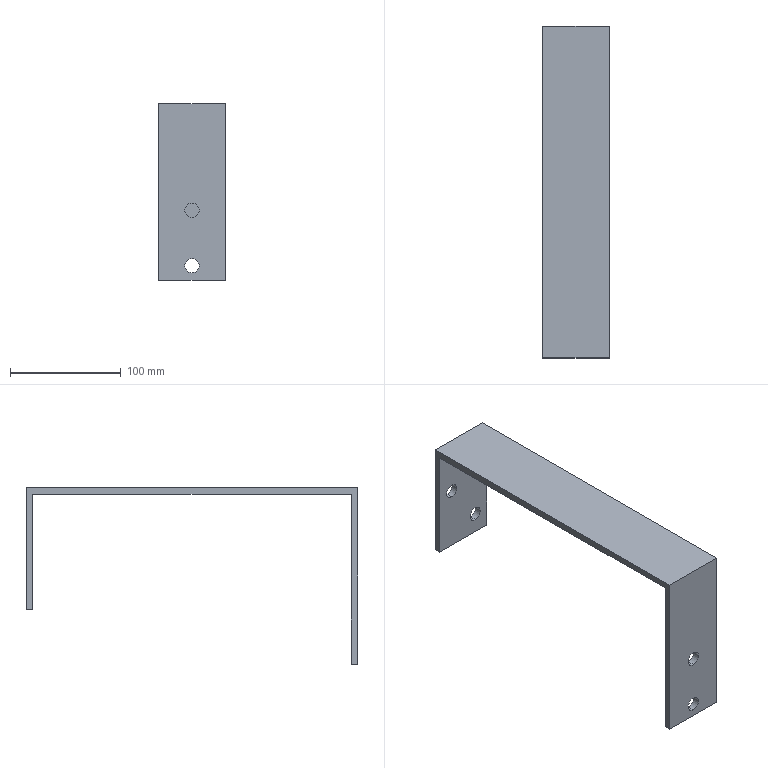Part | SolidWorks | features BaseBody 1 | 1 solid | 18 faces | box 60 x 299 x 159 mm | volume 196974 mm3 | plane 10 | cylinder 8 | commonest cylinder face diameters 13 x8
STEP:
#1=CARTESIAN_POINT('',(561.946,-3187.473,1586.471));
#2=VERTEX_POINT('',#1);
#3=CARTESIAN_POINT('',(561.946,-3187.473,1573.471));
#4=VERTEX_POINT('',#3);
#5=CARTESIAN_POINT('',(561.946,-3187.473,1579.971));
#6=DIRECTION('',(0.,-1.,0.));
#7=DIRECTION('',(0.,0.,-1.));
#8=AXIS2_PLACEMENT_3D('',#5,#6,#7);
#9=CIRCLE('',#8,6.5);
#10=EDGE_CURVE('',#2,#4,#9,.T.);
#11=ORIENTED_EDGE('',*,*,#10,.F.);
#12=CARTESIAN_POINT('',(561.946,-3193.473,1586.471));
#13=VERTEX_POINT('',#12);
#14=CARTESIAN_POINT('',(561.946,-3199.794,1586.471));
#15=DIRECTION('',(0.,-1.,0.));
#16=VECTOR('',#15,1000.);
#17=LINE('',#14,#16);
#18=EDGE_CURVE('',#2,#13,#17,.T.);
#19=ORIENTED_EDGE('',*,*,#18,.T.);
#20=CARTESIAN_POINT('',(561.946,-3193.473,1573.471));
#21=VERTEX_POINT('',#20);
#22=CARTESIAN_POINT('',(561.946,-3193.473,1579.971));
#23=DIRECTION('',(0.,1.,0.));
#24=DIRECTION('',(0.,0.,-1.));
#25=AXIS2_PLACEMENT_3D('',#22,#23,#24);
#26=CIRCLE('',#25,6.5);
#27=EDGE_CURVE('',#21,#13,#26,.T.);
#28=ORIENTED_EDGE('',*,*,#27,.F.);
#29=CARTESIAN_POINT('',(561.946,-3199.794,1573.471));
#30=DIRECTION('',(0.,-1.,0.));
#31=VECTOR('',#30,1000.);
#32=LINE('',#29,#31);
#33=EDGE_CURVE('',#4,#21,#32,.T.);
#34=ORIENTED_EDGE('',*,*,#33,.F.);
#35=EDGE_LOOP('',(#11,#19,#28,#34));
#36=FACE_OUTER_BOUND('',#35,.T.);
#37=CARTESIAN_POINT('',(561.946,-3199.794,1579.971));
#38=DIRECTION('',(0.,-1.,0.));
#39=DIRECTION('',(0.,0.,-1.));
#40=AXIS2_PLACEMENT_3D('',#37,#38,#39);
#41=CYLINDRICAL_SURFACE('',#40,6.5);
#42=ADVANCED_FACE('',(#36),#41,.F.);
#43=CARTESIAN_POINT('',(531.946,-3187.473,1626.471));
#44=VERTEX_POINT('',#43);
#45=CARTESIAN_POINT('',(531.946,-3187.473,1613.471));
#46=VERTEX_POINT('',#45);
#47=CARTESIAN_POINT('',(531.946,-3187.473,1619.971));
#48=DIRECTION('',(0.,-1.,0.));
#49=DIRECTION('',(0.,0.,-1.));
#50=AXIS2_PLACEMENT_3D('',#47,#48,#49);
#51=CIRCLE('',#50,6.5);
#52=EDGE_CURVE('',#44,#46,#51,.T.);
#53=ORIENTED_EDGE('',*,*,#52,.F.);
#54=CARTESIAN_POINT('',(531.946,-3193.473,1626.471));
#55=VERTEX_POINT('',#54);
#56=CARTESIAN_POINT('',(531.946,-3213.972,1626.471));
#57=DIRECTION('',(0.,-1.,0.));
#58=VECTOR('',#57,1000.);
#59=LINE('',#56,#58);
#60=EDGE_CURVE('',#44,#55,#59,.T.);
#61=ORIENTED_EDGE('',*,*,#60,.T.);
#62=CARTESIAN_POINT('',(531.946,-3193.473,1613.471));
#63=VERTEX_POINT('',#62);
#64=CARTESIAN_POINT('',(531.946,-3193.473,1619.971));
#65=DIRECTION('',(0.,1.,0.));
#66=DIRECTION('',(0.,0.,-1.));
#67=AXIS2_PLACEMENT_3D('',#64,#65,#66);
#68=CIRCLE('',#67,6.5);
#69=EDGE_CURVE('',#63,#55,#68,.T.);
#70=ORIENTED_EDGE('',*,*,#69,.F.);
#71=CARTESIAN_POINT('',(531.946,-3213.972,1613.471));
#72=DIRECTION('',(0.,-1.,0.));
#73=VECTOR('',#72,1000.);
#74=LINE('',#71,#73);
#75=EDGE_CURVE('',#46,#63,#74,.T.);
#76=ORIENTED_EDGE('',*,*,#75,.F.);
#77=EDGE_LOOP('',(#53,#61,#70,#76));
#78=FACE_OUTER_BOUND('',#77,.T.);
#79=CARTESIAN_POINT('',(531.946,-3213.972,1619.971));
#80=DIRECTION('',(0.,-1.,0.));
#81=DIRECTION('',(0.,0.,-1.));
#82=AXIS2_PLACEMENT_3D('',#79,#80,#81);
#83=CYLINDRICAL_SURFACE('',#82,6.5);
#84=ADVANCED_FACE('',(#78),#83,.F.);
#85=CARTESIAN_POINT('',(546.946,-3480.473,1580.471));
#86=VERTEX_POINT('',#85);
#87=CARTESIAN_POINT('',(546.946,-3480.473,1567.471));
#88=VERTEX_POINT('',#87);
#89=CARTESIAN_POINT('',(546.946,-3480.473,1573.971));
#90=DIRECTION('',(0.,-1.,0.));
#91=DIRECTION('',(0.,0.,-1.));
#92=AXIS2_PLACEMENT_3D('',#89,#90,#91);
#93=CIRCLE('',#92,6.5);
#94=EDGE_CURVE('',#86,#88,#93,.T.);
#95=ORIENTED_EDGE('',*,*,#94,.F.);
#96=CARTESIAN_POINT('',(546.946,-3486.473,1580.471));
#97=VERTEX_POINT('',#96);
#98=CARTESIAN_POINT('',(546.946,-3491.9,1580.471));
#99=DIRECTION('',(0.,-1.,0.));
#100=VECTOR('',#99,1000.);
#101=LINE('',#98,#100);
#102=EDGE_CURVE('',#86,#97,#101,.T.);
#103=ORIENTED_EDGE('',*,*,#102,.T.);
#104=CARTESIAN_POINT('',(546.946,-3486.473,1567.471));
#105=VERTEX_POINT('',#104);
#106=CARTESIAN_POINT('',(546.946,-3486.473,1573.971));
#107=DIRECTION('',(0.,1.,0.));
#108=DIRECTION('',(0.,0.,-1.));
#109=AXIS2_PLACEMENT_3D('',#106,#107,#108);
#110=CIRCLE('',#109,6.5);
#111=EDGE_CURVE('',#105,#97,#110,.T.);
#112=ORIENTED_EDGE('',*,*,#111,.F.);
#113=CARTESIAN_POINT('',(546.946,-3491.9,1567.471));
#114=DIRECTION('',(0.,-1.,0.));
#115=VECTOR('',#114,1000.);
#116=LINE('',#113,#115);
#117=EDGE_CURVE('',#88,#105,#116,.T.);
#118=ORIENTED_EDGE('',*,*,#117,.F.);
#119=EDGE_LOOP('',(#95,#103,#112,#118));
#120=FACE_OUTER_BOUND('',#119,.T.);
#121=CARTESIAN_POINT('',(546.946,-3491.9,1573.971));
#122=DIRECTION('',(0.,-1.,0.));
#123=DIRECTION('',(0.,0.,-1.));
#124=AXIS2_PLACEMENT_3D('',#121,#122,#123);
#125=CYLINDRICAL_SURFACE('',#124,6.5);
#126=ADVANCED_FACE('',(#120),#125,.F.);
#127=CARTESIAN_POINT('',(546.946,-3480.473,1530.471));
#128=VERTEX_POINT('',#127);
#129=CARTESIAN_POINT('',(546.946,-3480.473,1517.471));
#130=VERTEX_POINT('',#129);
#131=CARTESIAN_POINT('',(546.946,-3480.473,1523.971));
#132=DIRECTION('',(0.,-1.,0.));
#133=DIRECTION('',(0.,0.,-1.));
#134=AXIS2_PLACEMENT_3D('',#131,#132,#133);
#135=CIRCLE('',#134,6.5);
#136=EDGE_CURVE('',#128,#130,#135,.T.);
#137=ORIENTED_EDGE('',*,*,#136,.F.);
#138=CARTESIAN_POINT('',(546.946,-3486.473,1530.471));
#139=VERTEX_POINT('',#138);
#140=CARTESIAN_POINT('',(546.946,-3491.9,1530.471));
#141=DIRECTION('',(0.,-1.,0.));
#142=VECTOR('',#141,1000.);
#143=LINE('',#140,#142);
#144=EDGE_CURVE('',#128,#139,#143,.T.);
#145=ORIENTED_EDGE('',*,*,#144,.T.);
#146=CARTESIAN_POINT('',(546.946,-3486.473,1517.471));
#147=VERTEX_POINT('',#146);
#148=CARTESIAN_POINT('',(546.946,-3486.473,1523.971));
#149=DIRECTION('',(0.,1.,0.));
#150=DIRECTION('',(0.,0.,-1.));
#151=AXIS2_PLACEMENT_3D('',#148,#149,#150);
#152=CIRCLE('',#151,6.5);
#153=EDGE_CURVE('',#147,#139,#152,.T.);
#154=ORIENTED_EDGE('',*,*,#153,.F.);
#155=CARTESIAN_POINT('',(546.946,-3491.9,1517.471));
#156=DIRECTION('',(0.,-1.,0.));
#157=VECTOR('',#156,1000.);
#158=LINE('',#155,#157);
#159=EDGE_CURVE('',#130,#147,#158,.T.);
#160=ORIENTED_EDGE('',*,*,#159,.F.);
#161=EDGE_LOOP('',(#137,#145,#154,#160));
#162=FACE_OUTER_BOUND('',#161,.T.);
#163=CARTESIAN_POINT('',(546.946,-3491.9,1523.971));
#164=DIRECTION('',(0.,-1.,0.));
#165=DIRECTION('',(0.,0.,-1.));
#166=AXIS2_PLACEMENT_3D('',#163,#164,#165);
#167=CYLINDRICAL_SURFACE('',#166,6.5);
#168=ADVANCED_FACE('',(#162),#167,.F.);
#169=CARTESIAN_POINT('',(576.946,-3486.473,1669.971));
#170=VERTEX_POINT('',#169);
#171=CARTESIAN_POINT('',(576.946,-3187.473,1669.971));
#172=VERTEX_POINT('',#171);
#173=CARTESIAN_POINT('',(576.946,-3187.473,1669.971));
#174=DIRECTION('',(0.,1.,0.));
#175=VECTOR('',#174,1000.);
#176=LINE('',#173,#175);
#177=EDGE_CURVE('',#170,#172,#176,.T.);
#178=ORIENTED_EDGE('',*,*,#177,.T.);
#179=CARTESIAN_POINT('',(516.946,-3187.473,1669.971));
#180=VERTEX_POINT('',#179);
#181=CARTESIAN_POINT('',(576.946,-3187.473,1669.971));
#182=DIRECTION('',(-1.,0.,0.));
#183=VECTOR('',#182,1000.);
#184=LINE('',#181,#183);
#185=EDGE_CURVE('',#172,#180,#184,.T.);
#186=ORIENTED_EDGE('',*,*,#185,.T.);
#187=CARTESIAN_POINT('',(516.946,-3486.473,1669.971));
#188=VERTEX_POINT('',#187);
#189=CARTESIAN_POINT('',(516.946,-3187.473,1669.971));
#190=DIRECTION('',(0.,-1.,0.));
#191=VECTOR('',#190,1000.);
#192=LINE('',#189,#191);
#193=EDGE_CURVE('',#180,#188,#192,.T.);
#194=ORIENTED_EDGE('',*,*,#193,.T.);
#195=CARTESIAN_POINT('',(576.946,-3486.473,1669.971));
#196=DIRECTION('',(1.,0.,0.));
#197=VECTOR('',#196,1000.);
#198=LINE('',#195,#197);
#199=EDGE_CURVE('',#188,#170,#198,.T.);
#200=ORIENTED_EDGE('',*,*,#199,.T.);
#201=EDGE_LOOP('',(#178,#186,#194,#200));
#202=FACE_OUTER_BOUND('',#201,.T.);
#203=CARTESIAN_POINT('',(576.946,-3187.473,1669.971));
#204=DIRECTION('',(0.,0.,1.));
#205=DIRECTION('',(1.,0.,0.));
#206=AXIS2_PLACEMENT_3D('',#203,#204,#205);
#207=PLANE('',#206);
#208=ADVANCED_FACE('',(#202),#207,.T.);
#209=CARTESIAN_POINT('',(576.946,-3187.473,1559.971));
#210=VERTEX_POINT('',#209);
#211=CARTESIAN_POINT('',(576.946,-3187.473,1544.971));
#212=DIRECTION('',(0.,0.,-1.));
#213=VECTOR('',#212,1000.);
#214=LINE('',#211,#213);
#215=EDGE_CURVE('',#172,#210,#214,.T.);
#216=ORIENTED_EDGE('',*,*,#215,.T.);
#217=CARTESIAN_POINT('',(516.946,-3187.473,1559.971));
#218=VERTEX_POINT('',#217);
#219=CARTESIAN_POINT('',(576.946,-3187.473,1559.971));
#220=DIRECTION('',(-1.,0.,0.));
#221=VECTOR('',#220,1000.);
#222=LINE('',#219,#221);
#223=EDGE_CURVE('',#210,#218,#222,.T.);
#224=ORIENTED_EDGE('',*,*,#223,.T.);
#225=CARTESIAN_POINT('',(516.946,-3187.473,1544.971));
#226=DIRECTION('',(0.,0.,1.));
#227=VECTOR('',#226,1000.);
#228=LINE('',#225,#227);
#229=EDGE_CURVE('',#218,#180,#228,.T.);
#230=ORIENTED_EDGE('',*,*,#229,.T.);
#231=ORIENTED_EDGE('',*,*,#185,.F.);
#232=EDGE_LOOP('',(#216,#224,#230,#231));
#233=FACE_OUTER_BOUND('',#232,.T.);
#234=CARTESIAN_POINT('',(561.946,-3187.473,1579.971));
#235=DIRECTION('',(0.,-1.,0.));
#236=DIRECTION('',(0.,0.,-1.));
#237=AXIS2_PLACEMENT_3D('',#234,#235,#236);
#238=CIRCLE('',#237,6.5);
#239=EDGE_CURVE('',#4,#2,#238,.T.);
#240=ORIENTED_EDGE('',*,*,#239,.T.);
#241=ORIENTED_EDGE('',*,*,#10,.T.);
#242=EDGE_LOOP('',(#240,#241));
#243=FACE_BOUND('',#242,.T.);
#244=CARTESIAN_POINT('',(531.946,-3187.473,1619.971));
#245=DIRECTION('',(0.,-1.,0.));
#246=DIRECTION('',(0.,0.,-1.));
#247=AXIS2_PLACEMENT_3D('',#244,#245,#246);
#248=CIRCLE('',#247,6.5);
#249=EDGE_CURVE('',#46,#44,#248,.T.);
#250=ORIENTED_EDGE('',*,*,#249,.T.);
#251=ORIENTED_EDGE('',*,*,#52,.T.);
#252=EDGE_LOOP('',(#250,#251));
#253=FACE_BOUND('',#252,.T.);
#254=CARTESIAN_POINT('',(576.946,-3187.473,1544.971));
#255=DIRECTION('',(0.,1.,0.));
#256=DIRECTION('',(0.,0.,1.));
#257=AXIS2_PLACEMENT_3D('',#254,#255,#256);
#258=PLANE('',#257);
#259=ADVANCED_FACE('',(#233,#243,#253),#258,.T.);
#260=ORIENTED_EDGE('',*,*,#177,.F.);
#261=CARTESIAN_POINT('',(576.946,-3486.473,1510.971));
#262=VERTEX_POINT('',#261);
#263=CARTESIAN_POINT('',(576.946,-3486.473,1622.023));
#264=DIRECTION('',(0.,0.,-1.));
#265=VECTOR('',#264,1000.);
#266=LINE('',#263,#265);
#267=EDGE_CURVE('',#170,#262,#266,.T.);
#268=ORIENTED_EDGE('',*,*,#267,.T.);
#269=CARTESIAN_POINT('',(576.946,-3480.473,1510.971));
#270=VERTEX_POINT('',#269);
#271=CARTESIAN_POINT('',(576.946,-3346.079,1510.971));
#272=DIRECTION('',(0.,1.,0.));
#273=VECTOR('',#272,1000.);
#274=LINE('',#271,#273);
#275=EDGE_CURVE('',#262,#270,#274,.T.);
#276=ORIENTED_EDGE('',*,*,#275,.T.);
#277=CARTESIAN_POINT('',(576.946,-3480.473,1663.971));
#278=VERTEX_POINT('',#277);
#279=CARTESIAN_POINT('',(576.946,-3480.473,1622.023));
#280=DIRECTION('',(0.,0.,1.));
#281=VECTOR('',#280,1000.);
#282=LINE('',#279,#281);
#283=EDGE_CURVE('',#270,#278,#282,.T.);
#284=ORIENTED_EDGE('',*,*,#283,.T.);
#285=CARTESIAN_POINT('',(576.946,-3193.473,1663.971));
#286=VERTEX_POINT('',#285);
#287=CARTESIAN_POINT('',(576.946,-3346.079,1663.971));
#288=DIRECTION('',(0.,1.,0.));
#289=VECTOR('',#288,1000.);
#290=LINE('',#287,#289);
#291=EDGE_CURVE('',#278,#286,#290,.T.);
#292=ORIENTED_EDGE('',*,*,#291,.T.);
#293=CARTESIAN_POINT('',(576.946,-3193.473,1559.971));
#294=VERTEX_POINT('',#293);
#295=CARTESIAN_POINT('',(576.946,-3193.473,1622.023));
#296=DIRECTION('',(0.,0.,-1.));
#297=VECTOR('',#296,1000.);
#298=LINE('',#295,#297);
#299=EDGE_CURVE('',#286,#294,#298,.T.);
#300=ORIENTED_EDGE('',*,*,#299,.T.);
#301=CARTESIAN_POINT('',(576.946,-3346.079,1559.971));
#302=DIRECTION('',(0.,1.,0.));
#303=VECTOR('',#302,1000.);
#304=LINE('',#301,#303);
#305=EDGE_CURVE('',#294,#210,#304,.T.);
#306=ORIENTED_EDGE('',*,*,#305,.T.);
#307=ORIENTED_EDGE('',*,*,#215,.F.);
#308=EDGE_LOOP('',(#260,#268,#276,#284,#292,#300,#306,#307));
#309=FACE_OUTER_BOUND('',#308,.T.);
#310=CARTESIAN_POINT('',(576.946,-3346.079,1622.023));
#311=DIRECTION('',(1.,0.,0.));
#312=DIRECTION('',(0.,0.,-1.));
#313=AXIS2_PLACEMENT_3D('',#310,#311,#312);
#314=PLANE('',#313);
#315=ADVANCED_FACE('',(#309),#314,.T.);
#316=ORIENTED_EDGE('',*,*,#267,.F.);
#317=ORIENTED_EDGE('',*,*,#199,.F.);
#318=CARTESIAN_POINT('',(516.946,-3486.473,1510.971));
#319=VERTEX_POINT('',#318);
#320=CARTESIAN_POINT('',(516.946,-3486.473,1654.971));
#321=DIRECTION('',(0.,0.,-1.));
#322=VECTOR('',#321,1000.);
#323=LINE('',#320,#322);
#324=EDGE_CURVE('',#188,#319,#323,.T.);
#325=ORIENTED_EDGE('',*,*,#324,.T.);
#326=CARTESIAN_POINT('',(576.946,-3486.473,1510.971));
#327=DIRECTION('',(1.,0.,0.));
#328=VECTOR('',#327,1000.);
#329=LINE('',#326,#328);
#330=EDGE_CURVE('',#319,#262,#329,.T.);
#331=ORIENTED_EDGE('',*,*,#330,.T.);
#332=EDGE_LOOP('',(#316,#317,#325,#331));
#333=FACE_OUTER_BOUND('',#332,.T.);
#334=ORIENTED_EDGE('',*,*,#111,.T.);
#335=CARTESIAN_POINT('',(546.946,-3486.473,1573.971));
#336=DIRECTION('',(0.,1.,0.));
#337=DIRECTION('',(0.,0.,-1.));
#338=AXIS2_PLACEMENT_3D('',#335,#336,#337);
#339=CIRCLE('',#338,6.5);
#340=EDGE_CURVE('',#97,#105,#339,.T.);
#341=ORIENTED_EDGE('',*,*,#340,.T.);
#342=EDGE_LOOP('',(#334,#341));
#343=FACE_BOUND('',#342,.T.);
#344=ORIENTED_EDGE('',*,*,#153,.T.);
#345=CARTESIAN_POINT('',(546.946,-3486.473,1523.971));
#346=DIRECTION('',(0.,1.,0.));
#347=DIRECTION('',(0.,0.,-1.));
#348=AXIS2_PLACEMENT_3D('',#345,#346,#347);
#349=CIRCLE('',#348,6.5);
#350=EDGE_CURVE('',#139,#147,#349,.T.);
#351=ORIENTED_EDGE('',*,*,#350,.T.);
#352=EDGE_LOOP('',(#344,#351));
#353=FACE_BOUND('',#352,.T.);
#354=CARTESIAN_POINT('',(576.946,-3486.473,1654.971));
#355=DIRECTION('',(0.,-1.,0.));
#356=DIRECTION('',(0.,0.,-1.));
#357=AXIS2_PLACEMENT_3D('',#354,#355,#356);
#358=PLANE('',#357);
#359=ADVANCED_FACE('',(#333,#343,#353),#358,.T.);
#360=CARTESIAN_POINT('',(516.946,-3480.473,1510.971));
#361=VERTEX_POINT('',#360);
#362=CARTESIAN_POINT('',(516.946,-3346.079,1510.971));
#363=DIRECTION('',(0.,1.,0.));
#364=VECTOR('',#363,1000.);
#365=LINE('',#362,#364);
#366=EDGE_CURVE('',#319,#361,#365,.T.);
#367=ORIENTED_EDGE('',*,*,#366,.F.);
#368=ORIENTED_EDGE('',*,*,#324,.F.);
#369=ORIENTED_EDGE('',*,*,#193,.F.);
#370=ORIENTED_EDGE('',*,*,#229,.F.);
#371=CARTESIAN_POINT('',(516.946,-3193.473,1559.971));
#372=VERTEX_POINT('',#371);
#373=CARTESIAN_POINT('',(516.946,-3346.079,1559.971));
#374=DIRECTION('',(0.,1.,0.));
#375=VECTOR('',#374,1000.);
#376=LINE('',#373,#375);
#377=EDGE_CURVE('',#372,#218,#376,.T.);
#378=ORIENTED_EDGE('',*,*,#377,.F.);
#379=CARTESIAN_POINT('',(516.946,-3193.473,1663.971));
#380=VERTEX_POINT('',#379);
#381=CARTESIAN_POINT('',(516.946,-3193.473,1652.023));
#382=DIRECTION('',(0.,0.,-1.));
#383=VECTOR('',#382,1000.);
#384=LINE('',#381,#383);
#385=EDGE_CURVE('',#380,#372,#384,.T.);
#386=ORIENTED_EDGE('',*,*,#385,.F.);
#387=CARTESIAN_POINT('',(516.946,-3480.473,1663.971));
#388=VERTEX_POINT('',#387);
#389=CARTESIAN_POINT('',(516.946,-3346.079,1663.971));
#390=DIRECTION('',(0.,1.,0.));
#391=VECTOR('',#390,1000.);
#392=LINE('',#389,#391);
#393=EDGE_CURVE('',#388,#380,#392,.T.);
#394=ORIENTED_EDGE('',*,*,#393,.F.);
#395=CARTESIAN_POINT('',(516.946,-3480.473,1652.023));
#396=DIRECTION('',(0.,0.,1.));
#397=VECTOR('',#396,1000.);
#398=LINE('',#395,#397);
#399=EDGE_CURVE('',#361,#388,#398,.T.);
#400=ORIENTED_EDGE('',*,*,#399,.F.);
#401=EDGE_LOOP('',(#367,#368,#369,#370,#378,#386,#394,#400));
#402=FACE_OUTER_BOUND('',#401,.T.);
#403=CARTESIAN_POINT('',(516.946,-3346.079,1652.023));
#404=DIRECTION('',(1.,0.,0.));
#405=DIRECTION('',(0.,0.,-1.));
#406=AXIS2_PLACEMENT_3D('',#403,#404,#405);
#407=PLANE('',#406);
#408=ADVANCED_FACE('',(#402),#407,.F.);
#409=ORIENTED_EDGE('',*,*,#305,.F.);
#410=CARTESIAN_POINT('',(576.946,-3193.473,1559.971));
#411=DIRECTION('',(-1.,0.,0.));
#412=VECTOR('',#411,1000.);
#413=LINE('',#410,#412);
#414=EDGE_CURVE('',#294,#372,#413,.T.);
#415=ORIENTED_EDGE('',*,*,#414,.T.);
#416=ORIENTED_EDGE('',*,*,#377,.T.);
#417=ORIENTED_EDGE('',*,*,#223,.F.);
#418=EDGE_LOOP('',(#409,#415,#416,#417));
#419=FACE_OUTER_BOUND('',#418,.T.);
#420=CARTESIAN_POINT('',(576.946,-3193.473,1559.971));
#421=DIRECTION('',(0.,0.,-1.));
#422=DIRECTION('',(-1.,0.,0.));
#423=AXIS2_PLACEMENT_3D('',#420,#421,#422);
#424=PLANE('',#423);
#425=ADVANCED_FACE('',(#419),#424,.T.);
#426=ORIENTED_EDGE('',*,*,#18,.F.);
#427=ORIENTED_EDGE('',*,*,#239,.F.);
#428=ORIENTED_EDGE('',*,*,#33,.T.);
#429=CARTESIAN_POINT('',(561.946,-3193.473,1579.971));
#430=DIRECTION('',(0.,1.,0.));
#431=DIRECTION('',(0.,0.,-1.));
#432=AXIS2_PLACEMENT_3D('',#429,#430,#431);
#433=CIRCLE('',#432,6.5);
#434=EDGE_CURVE('',#13,#21,#433,.T.);
#435=ORIENTED_EDGE('',*,*,#434,.F.);
#436=EDGE_LOOP('',(#426,#427,#428,#435));
#437=FACE_OUTER_BOUND('',#436,.T.);
#438=CARTESIAN_POINT('',(561.946,-3199.794,1579.971));
#439=DIRECTION('',(0.,-1.,0.));
#440=DIRECTION('',(0.,0.,-1.));
#441=AXIS2_PLACEMENT_3D('',#438,#439,#440);
#442=CYLINDRICAL_SURFACE('',#441,6.5);
#443=ADVANCED_FACE('',(#437),#442,.F.);
#444=ORIENTED_EDGE('',*,*,#60,.F.);
#445=ORIENTED_EDGE('',*,*,#249,.F.);
#446=ORIENTED_EDGE('',*,*,#75,.T.);
#447=CARTESIAN_POINT('',(531.946,-3193.473,1619.971));
#448=DIRECTION('',(0.,1.,0.));
#449=DIRECTION('',(0.,0.,-1.));
#450=AXIS2_PLACEMENT_3D('',#447,#448,#449);
#451=CIRCLE('',#450,6.5);
#452=EDGE_CURVE('',#55,#63,#451,.T.);
#453=ORIENTED_EDGE('',*,*,#452,.F.);
#454=EDGE_LOOP('',(#444,#445,#446,#453));
#455=FACE_OUTER_BOUND('',#454,.T.);
#456=CARTESIAN_POINT('',(531.946,-3213.972,1619.971));
#457=DIRECTION('',(0.,-1.,0.));
#458=DIRECTION('',(0.,0.,-1.));
#459=AXIS2_PLACEMENT_3D('',#456,#457,#458);
#460=CYLINDRICAL_SURFACE('',#459,6.5);
#461=ADVANCED_FACE('',(#455),#460,.F.);
#462=ORIENTED_EDGE('',*,*,#299,.F.);
#463=CARTESIAN_POINT('',(576.946,-3193.473,1663.971));
#464=DIRECTION('',(-1.,0.,0.));
#465=VECTOR('',#464,1000.);
#466=LINE('',#463,#465);
#467=EDGE_CURVE('',#286,#380,#466,.T.);
#468=ORIENTED_EDGE('',*,*,#467,.T.);
#469=ORIENTED_EDGE('',*,*,#385,.T.);
#470=ORIENTED_EDGE('',*,*,#414,.F.);
#471=EDGE_LOOP('',(#462,#468,#469,#470));
#472=FACE_OUTER_BOUND('',#471,.T.);
#473=ORIENTED_EDGE('',*,*,#27,.T.);
#474=ORIENTED_EDGE('',*,*,#434,.T.);
#475=EDGE_LOOP('',(#473,#474));
#476=FACE_BOUND('',#475,.T.);
#477=ORIENTED_EDGE('',*,*,#69,.T.);
#478=ORIENTED_EDGE('',*,*,#452,.T.);
#479=EDGE_LOOP('',(#477,#478));
#480=FACE_BOUND('',#479,.T.);
#481=CARTESIAN_POINT('',(576.946,-3193.473,1663.971));
#482=DIRECTION('',(0.,-1.,0.));
#483=DIRECTION('',(0.,0.,-1.));
#484=AXIS2_PLACEMENT_3D('',#481,#482,#483);
#485=PLANE('',#484);
#486=ADVANCED_FACE('',(#472,#476,#480),#485,.T.);
#487=ORIENTED_EDGE('',*,*,#291,.F.);
#488=CARTESIAN_POINT('',(576.946,-3480.473,1663.971));
#489=DIRECTION('',(-1.,0.,0.));
#490=VECTOR('',#489,1000.);
#491=LINE('',#488,#490);
#492=EDGE_CURVE('',#278,#388,#491,.T.);
#493=ORIENTED_EDGE('',*,*,#492,.T.);
#494=ORIENTED_EDGE('',*,*,#393,.T.);
#495=ORIENTED_EDGE('',*,*,#467,.F.);
#496=EDGE_LOOP('',(#487,#493,#494,#495));
#497=FACE_OUTER_BOUND('',#496,.T.);
#498=CARTESIAN_POINT('',(576.946,-3480.473,1663.971));
#499=DIRECTION('',(0.,0.,-1.));
#500=DIRECTION('',(-1.,0.,0.));
#501=AXIS2_PLACEMENT_3D('',#498,#499,#500);
#502=PLANE('',#501);
#503=ADVANCED_FACE('',(#497),#502,.T.);
#504=ORIENTED_EDGE('',*,*,#283,.F.);
#505=CARTESIAN_POINT('',(576.946,-3480.473,1510.971));
#506=DIRECTION('',(-1.,0.,0.));
#507=VECTOR('',#506,1000.);
#508=LINE('',#505,#507);
#509=EDGE_CURVE('',#270,#361,#508,.T.);
#510=ORIENTED_EDGE('',*,*,#509,.T.);
#511=ORIENTED_EDGE('',*,*,#399,.T.);
#512=ORIENTED_EDGE('',*,*,#492,.F.);
#513=EDGE_LOOP('',(#504,#510,#511,#512));
#514=FACE_OUTER_BOUND('',#513,.T.);
#515=CARTESIAN_POINT('',(546.946,-3480.473,1573.971));
#516=DIRECTION('',(0.,-1.,0.));
#517=DIRECTION('',(0.,0.,-1.));
#518=AXIS2_PLACEMENT_3D('',#515,#516,#517);
#519=CIRCLE('',#518,6.5);
#520=EDGE_CURVE('',#88,#86,#519,.T.);
#521=ORIENTED_EDGE('',*,*,#520,.T.);
#522=ORIENTED_EDGE('',*,*,#94,.T.);
#523=EDGE_LOOP('',(#521,#522));
#524=FACE_BOUND('',#523,.T.);
#525=CARTESIAN_POINT('',(546.946,-3480.473,1523.971));
#526=DIRECTION('',(0.,-1.,0.));
#527=DIRECTION('',(0.,0.,-1.));
#528=AXIS2_PLACEMENT_3D('',#525,#526,#527);
#529=CIRCLE('',#528,6.5);
#530=EDGE_CURVE('',#130,#128,#529,.T.);
#531=ORIENTED_EDGE('',*,*,#530,.T.);
#532=ORIENTED_EDGE('',*,*,#136,.T.);
#533=EDGE_LOOP('',(#531,#532));
#534=FACE_BOUND('',#533,.T.);
#535=CARTESIAN_POINT('',(576.946,-3480.473,1510.971));
#536=DIRECTION('',(0.,1.,0.));
#537=DIRECTION('',(0.,0.,1.));
#538=AXIS2_PLACEMENT_3D('',#535,#536,#537);
#539=PLANE('',#538);
#540=ADVANCED_FACE('',(#514,#524,#534),#539,.T.);
#541=ORIENTED_EDGE('',*,*,#275,.F.);
#542=ORIENTED_EDGE('',*,*,#330,.F.);
#543=ORIENTED_EDGE('',*,*,#366,.T.);
#544=ORIENTED_EDGE('',*,*,#509,.F.);
#545=EDGE_LOOP('',(#541,#542,#543,#544));
#546=FACE_OUTER_BOUND('',#545,.T.);
#547=CARTESIAN_POINT('',(576.946,-3486.473,1510.971));
#548=DIRECTION('',(0.,0.,-1.));
#549=DIRECTION('',(-1.,0.,0.));
#550=AXIS2_PLACEMENT_3D('',#547,#548,#549);
#551=PLANE('',#550);
#552=ADVANCED_FACE('',(#546),#551,.T.);
#553=ORIENTED_EDGE('',*,*,#102,.F.);
#554=ORIENTED_EDGE('',*,*,#520,.F.);
#555=ORIENTED_EDGE('',*,*,#117,.T.);
#556=ORIENTED_EDGE('',*,*,#340,.F.);
#557=EDGE_LOOP('',(#553,#554,#555,#556));
#558=FACE_OUTER_BOUND('',#557,.T.);
#559=CARTESIAN_POINT('',(546.946,-3491.9,1573.971));
#560=DIRECTION('',(0.,-1.,0.));
#561=DIRECTION('',(0.,0.,-1.));
#562=AXIS2_PLACEMENT_3D('',#559,#560,#561);
#563=CYLINDRICAL_SURFACE('',#562,6.5);
#564=ADVANCED_FACE('',(#558),#563,.F.);
#565=ORIENTED_EDGE('',*,*,#144,.F.);
#566=ORIENTED_EDGE('',*,*,#530,.F.);
#567=ORIENTED_EDGE('',*,*,#159,.T.);
#568=ORIENTED_EDGE('',*,*,#350,.F.);
#569=EDGE_LOOP('',(#565,#566,#567,#568));
#570=FACE_OUTER_BOUND('',#569,.T.);
#571=CARTESIAN_POINT('',(546.946,-3491.9,1523.971));
#572=DIRECTION('',(0.,-1.,0.));
#573=DIRECTION('',(0.,0.,-1.));
#574=AXIS2_PLACEMENT_3D('',#571,#572,#573);
#575=CYLINDRICAL_SURFACE('',#574,6.5);
#576=ADVANCED_FACE('',(#570),#575,.F.);
#577=CLOSED_SHELL('',(#42,#84,#126,#168,#208,#259,#315,#359,#408,#425,#443,#461,#486,#503,#540,#552,#564,#576));
#578=MANIFOLD_SOLID_BREP('',#577);
#579=CARTESIAN_POINT('',(0.,0.,0.));
#580=DIRECTION('',(0.,0.,1.));
#581=DIRECTION('',(1.,0.,0.));
#582=AXIS2_PLACEMENT_3D('',#579,#580,#581);
#583=(LENGTH_UNIT()NAMED_UNIT(*)SI_UNIT(.MILLI.,.METRE.));
#584=UNCERTAINTY_MEASURE_WITH_UNIT(LENGTH_MEASURE(0.00001),#583,'','');
#585=(NAMED_UNIT(*)PLANE_ANGLE_UNIT()SI_UNIT($,.RADIAN.));
#586=(NAMED_UNIT(*)SI_UNIT($,.STERADIAN.)SOLID_ANGLE_UNIT());
#587=(GEOMETRIC_REPRESENTATION_CONTEXT(3)GLOBAL_UNCERTAINTY_ASSIGNED_CONTEXT((#584))GLOBAL_UNIT_ASSIGNED_CONTEXT((#583,#585,#586))REPRESENTATION_CONTEXT('',''));
#588=ADVANCED_BREP_SHAPE_REPRESENTATION('',(#578,#582),#587);